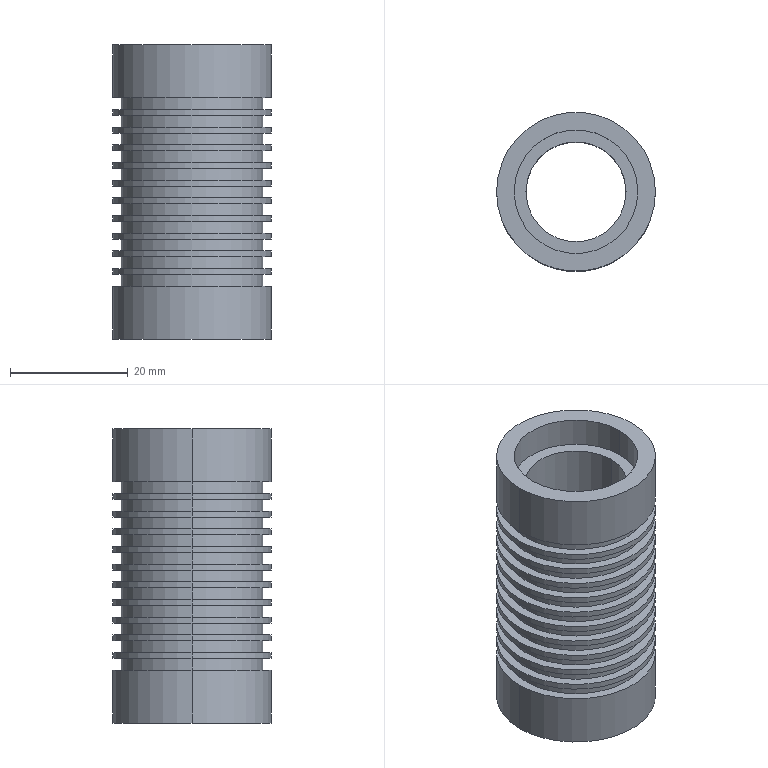Part | SolidWorks | features MirrorPattern 2, Extrusion 1, ICE 1, LPattern 1, RevCut 1 | 1 solid | 78 faces | box 27 x 27 x 50 mm | volume 13441 mm3 | cylinder 52 | plane 26 | commonest cylinder face diameters 27 x24 24 x22 21 x4 17 x2